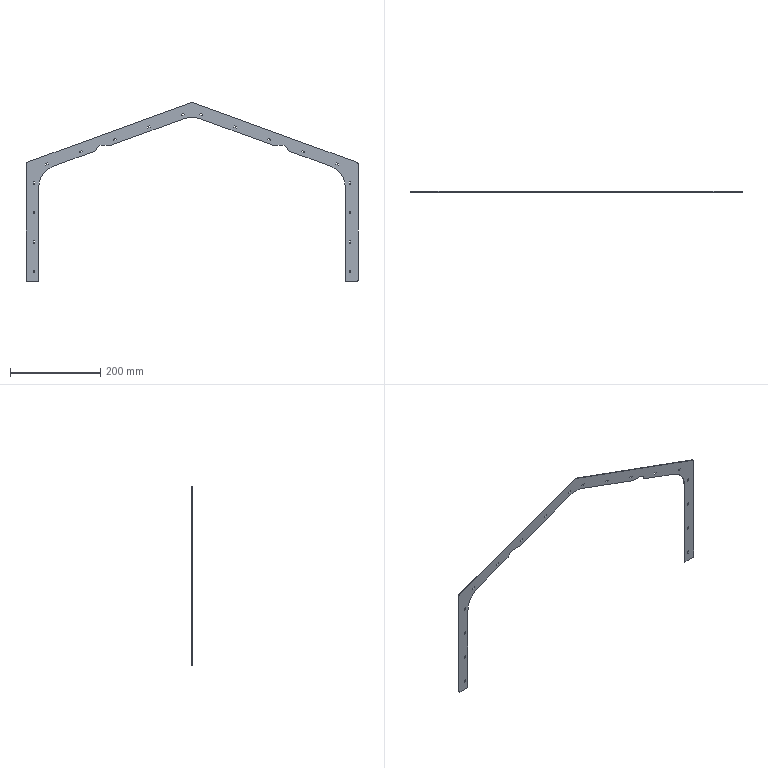Part | NX | features solid 2 | 1 solid | 100 faces | box 734 x 2 x 396.257 mm | volume 70071 mm3 | plane 90 | cylinder 10 | commonest cylinder face diameters 6 x5 100 x3 30 x2